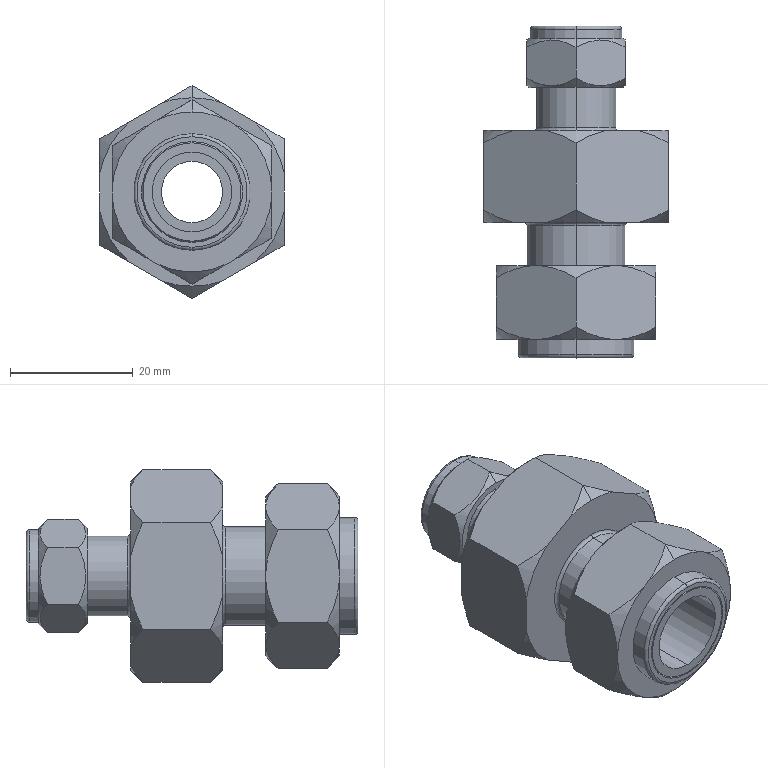Part | SolidWorks | features ICE 8, Fillet 3, Extrusion 1, RevCut 1 | 3 solids | 85 faces | box 30 x 54 x 34.641 mm | volume 18354 mm3 | cone 32 | plane 29 | cylinder 16 | torus 8 | commonest cylinder face diameters 13 x4 10 x2 13.2 x2 15 x2 16 x2 16.4 x2